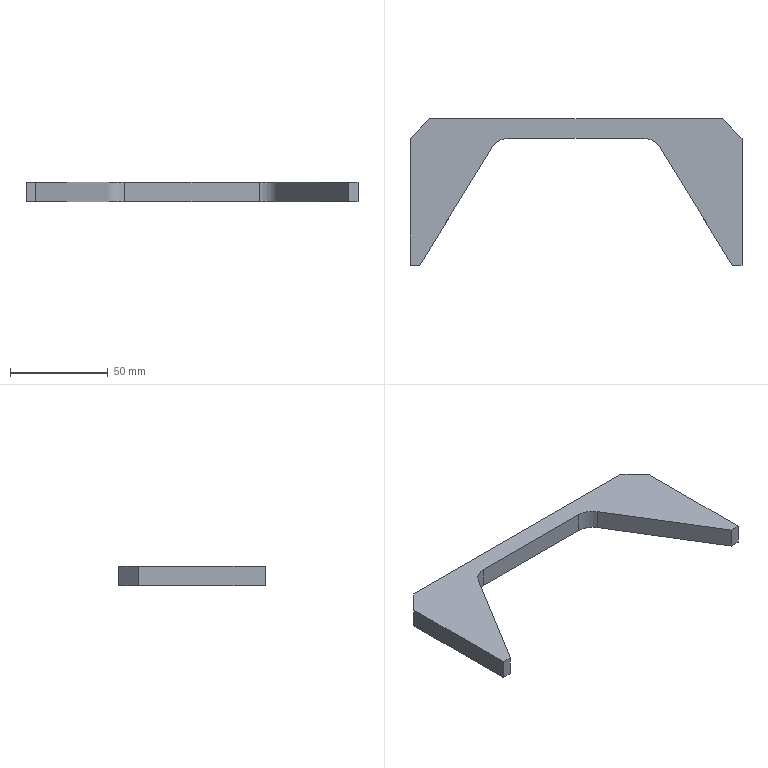Part | SolidWorks | features Chamfer 1, Extrusion 1 | 1 solid | 14 faces | box 170 x 75 x 10 mm | volume 48537 mm3 | plane 12 | cylinder 2 | commonest cylinder face diameters 20 x2
STEP:
#1=CARTESIAN_POINT('',(-85.,65.,5.));
#2=VERTEX_POINT('',#1);
#3=CARTESIAN_POINT('',(-85.,0.,5.));
#4=VERTEX_POINT('',#3);
#5=CARTESIAN_POINT('',(-85.,75.,5.));
#6=DIRECTION('',(0.,-1.,0.));
#7=VECTOR('',#6,1000.);
#8=LINE('',#5,#7);
#9=EDGE_CURVE('',#2,#4,#8,.T.);
#10=ORIENTED_EDGE('',*,*,#9,.F.);
#11=CARTESIAN_POINT('',(-85.,65.,-5.));
#12=VERTEX_POINT('',#11);
#13=CARTESIAN_POINT('',(-85.,65.,5.));
#14=DIRECTION('',(0.,0.,-1.));
#15=VECTOR('',#14,1000.);
#16=LINE('',#13,#15);
#17=EDGE_CURVE('',#2,#12,#16,.T.);
#18=ORIENTED_EDGE('',*,*,#17,.T.);
#19=CARTESIAN_POINT('',(-85.,0.,-5.));
#20=VERTEX_POINT('',#19);
#21=CARTESIAN_POINT('',(-85.,75.,-5.));
#22=DIRECTION('',(0.,-1.,0.));
#23=VECTOR('',#22,1000.);
#24=LINE('',#21,#23);
#25=EDGE_CURVE('',#12,#20,#24,.T.);
#26=ORIENTED_EDGE('',*,*,#25,.T.);
#27=CARTESIAN_POINT('',(-85.,0.,5.));
#28=DIRECTION('',(0.,0.,-1.));
#29=VECTOR('',#28,1000.);
#30=LINE('',#27,#29);
#31=EDGE_CURVE('',#4,#20,#30,.T.);
#32=ORIENTED_EDGE('',*,*,#31,.F.);
#33=EDGE_LOOP('',(#10,#18,#26,#32));
#34=FACE_OUTER_BOUND('',#33,.T.);
#35=CARTESIAN_POINT('',(-85.,75.,5.));
#36=DIRECTION('',(1.,0.,0.));
#37=DIRECTION('',(0.,0.,-1.));
#38=AXIS2_PLACEMENT_3D('',#35,#36,#37);
#39=PLANE('',#38);
#40=ADVANCED_FACE('',(#34),#39,.F.);
#41=CARTESIAN_POINT('',(-80.,0.,-5.));
#42=VERTEX_POINT('',#41);
#43=CARTESIAN_POINT('',(-85.,0.,-5.));
#44=DIRECTION('',(1.,0.,0.));
#45=VECTOR('',#44,1000.);
#46=LINE('',#43,#45);
#47=EDGE_CURVE('',#20,#42,#46,.T.);
#48=ORIENTED_EDGE('',*,*,#47,.T.);
#49=CARTESIAN_POINT('',(-80.,0.,5.));
#50=VERTEX_POINT('',#49);
#51=CARTESIAN_POINT('',(-80.,0.,5.));
#52=DIRECTION('',(0.,0.,-1.));
#53=VECTOR('',#52,1000.);
#54=LINE('',#51,#53);
#55=EDGE_CURVE('',#50,#42,#54,.T.);
#56=ORIENTED_EDGE('',*,*,#55,.F.);
#57=CARTESIAN_POINT('',(-85.,0.,5.));
#58=DIRECTION('',(1.,0.,0.));
#59=VECTOR('',#58,1000.);
#60=LINE('',#57,#59);
#61=EDGE_CURVE('',#4,#50,#60,.T.);
#62=ORIENTED_EDGE('',*,*,#61,.F.);
#63=ORIENTED_EDGE('',*,*,#31,.T.);
#64=EDGE_LOOP('',(#48,#56,#62,#63));
#65=FACE_OUTER_BOUND('',#64,.T.);
#66=CARTESIAN_POINT('',(-85.,0.,5.));
#67=DIRECTION('',(0.,1.,0.));
#68=DIRECTION('',(0.,0.,1.));
#69=AXIS2_PLACEMENT_3D('',#66,#67,#68);
#70=PLANE('',#69);
#71=ADVANCED_FACE('',(#65),#70,.F.);
#72=CARTESIAN_POINT('',(-43.022,60.232,-5.));
#73=VERTEX_POINT('',#72);
#74=CARTESIAN_POINT('',(-80.,0.,-5.));
#75=DIRECTION('',(0.5232,0.8522,0.));
#76=VECTOR('',#75,1000.);
#77=LINE('',#74,#76);
#78=EDGE_CURVE('',#42,#73,#77,.T.);
#79=ORIENTED_EDGE('',*,*,#78,.T.);
#80=CARTESIAN_POINT('',(-43.022,60.232,5.));
#81=VERTEX_POINT('',#80);
#82=CARTESIAN_POINT('',(-43.022,60.232,5.));
#83=DIRECTION('',(0.,0.,-1.));
#84=VECTOR('',#83,1000.);
#85=LINE('',#82,#84);
#86=EDGE_CURVE('',#81,#73,#85,.T.);
#87=ORIENTED_EDGE('',*,*,#86,.F.);
#88=CARTESIAN_POINT('',(-80.,0.,5.));
#89=DIRECTION('',(0.5232,0.8522,0.));
#90=VECTOR('',#89,1000.);
#91=LINE('',#88,#90);
#92=EDGE_CURVE('',#50,#81,#91,.T.);
#93=ORIENTED_EDGE('',*,*,#92,.F.);
#94=ORIENTED_EDGE('',*,*,#55,.T.);
#95=EDGE_LOOP('',(#79,#87,#93,#94));
#96=FACE_OUTER_BOUND('',#95,.T.);
#97=CARTESIAN_POINT('',(-80.,0.,5.));
#98=DIRECTION('',(-0.8522,0.5232,0.));
#99=DIRECTION('',(-0.5232,-0.8522,0.));
#100=AXIS2_PLACEMENT_3D('',#97,#98,#99);
#101=PLANE('',#100);
#102=ADVANCED_FACE('',(#96),#101,.F.);
#103=CARTESIAN_POINT('',(-34.5,65.,-5.));
#104=VERTEX_POINT('',#103);
#105=CARTESIAN_POINT('',(-34.5,55.,-5.));
#106=DIRECTION('',(0.,0.,-1.));
#107=DIRECTION('',(-1.,0.,0.));
#108=AXIS2_PLACEMENT_3D('',#105,#106,#107);
#109=CIRCLE('',#108,10.);
#110=EDGE_CURVE('',#73,#104,#109,.T.);
#111=ORIENTED_EDGE('',*,*,#110,.T.);
#112=CARTESIAN_POINT('',(-34.5,65.,5.));
#113=VERTEX_POINT('',#112);
#114=CARTESIAN_POINT('',(-34.5,65.,5.));
#115=DIRECTION('',(0.,0.,-1.));
#116=VECTOR('',#115,1000.);
#117=LINE('',#114,#116);
#118=EDGE_CURVE('',#113,#104,#117,.T.);
#119=ORIENTED_EDGE('',*,*,#118,.F.);
#120=CARTESIAN_POINT('',(-34.5,55.,5.));
#121=DIRECTION('',(0.,0.,-1.));
#122=DIRECTION('',(-1.,0.,0.));
#123=AXIS2_PLACEMENT_3D('',#120,#121,#122);
#124=CIRCLE('',#123,10.);
#125=EDGE_CURVE('',#81,#113,#124,.T.);
#126=ORIENTED_EDGE('',*,*,#125,.F.);
#127=ORIENTED_EDGE('',*,*,#86,.T.);
#128=EDGE_LOOP('',(#111,#119,#126,#127));
#129=FACE_OUTER_BOUND('',#128,.T.);
#130=CARTESIAN_POINT('',(-34.5,55.,5.));
#131=DIRECTION('',(0.,0.,-1.));
#132=DIRECTION('',(-1.,0.,0.));
#133=AXIS2_PLACEMENT_3D('',#130,#131,#132);
#134=CYLINDRICAL_SURFACE('',#133,10.);
#135=ADVANCED_FACE('',(#129),#134,.F.);
#136=CARTESIAN_POINT('',(34.5,65.,-5.));
#137=VERTEX_POINT('',#136);
#138=CARTESIAN_POINT('',(-34.5,65.,-5.));
#139=DIRECTION('',(1.,0.,0.));
#140=VECTOR('',#139,1000.);
#141=LINE('',#138,#140);
#142=EDGE_CURVE('',#104,#137,#141,.T.);
#143=ORIENTED_EDGE('',*,*,#142,.T.);
#144=CARTESIAN_POINT('',(34.5,65.,5.));
#145=VERTEX_POINT('',#144);
#146=CARTESIAN_POINT('',(34.5,65.,5.));
#147=DIRECTION('',(0.,0.,-1.));
#148=VECTOR('',#147,1000.);
#149=LINE('',#146,#148);
#150=EDGE_CURVE('',#145,#137,#149,.T.);
#151=ORIENTED_EDGE('',*,*,#150,.F.);
#152=CARTESIAN_POINT('',(-34.5,65.,5.));
#153=DIRECTION('',(1.,0.,0.));
#154=VECTOR('',#153,1000.);
#155=LINE('',#152,#154);
#156=EDGE_CURVE('',#113,#145,#155,.T.);
#157=ORIENTED_EDGE('',*,*,#156,.F.);
#158=ORIENTED_EDGE('',*,*,#118,.T.);
#159=EDGE_LOOP('',(#143,#151,#157,#158));
#160=FACE_OUTER_BOUND('',#159,.T.);
#161=CARTESIAN_POINT('',(-34.5,65.,5.));
#162=DIRECTION('',(0.,1.,0.));
#163=DIRECTION('',(0.,0.,1.));
#164=AXIS2_PLACEMENT_3D('',#161,#162,#163);
#165=PLANE('',#164);
#166=ADVANCED_FACE('',(#160),#165,.F.);
#167=CARTESIAN_POINT('',(43.022,60.232,-5.));
#168=VERTEX_POINT('',#167);
#169=CARTESIAN_POINT('',(34.5,55.,-5.));
#170=DIRECTION('',(0.,0.,-1.));
#171=DIRECTION('',(1.,0.,0.));
#172=AXIS2_PLACEMENT_3D('',#169,#170,#171);
#173=CIRCLE('',#172,10.);
#174=EDGE_CURVE('',#137,#168,#173,.T.);
#175=ORIENTED_EDGE('',*,*,#174,.T.);
#176=CARTESIAN_POINT('',(43.022,60.232,5.));
#177=VERTEX_POINT('',#176);
#178=CARTESIAN_POINT('',(43.022,60.232,5.));
#179=DIRECTION('',(0.,0.,-1.));
#180=VECTOR('',#179,1000.);
#181=LINE('',#178,#180);
#182=EDGE_CURVE('',#177,#168,#181,.T.);
#183=ORIENTED_EDGE('',*,*,#182,.F.);
#184=CARTESIAN_POINT('',(34.5,55.,5.));
#185=DIRECTION('',(0.,0.,-1.));
#186=DIRECTION('',(1.,0.,0.));
#187=AXIS2_PLACEMENT_3D('',#184,#185,#186);
#188=CIRCLE('',#187,10.);
#189=EDGE_CURVE('',#145,#177,#188,.T.);
#190=ORIENTED_EDGE('',*,*,#189,.F.);
#191=ORIENTED_EDGE('',*,*,#150,.T.);
#192=EDGE_LOOP('',(#175,#183,#190,#191));
#193=FACE_OUTER_BOUND('',#192,.T.);
#194=CARTESIAN_POINT('',(34.5,55.,5.));
#195=DIRECTION('',(0.,0.,-1.));
#196=DIRECTION('',(-1.,0.,0.));
#197=AXIS2_PLACEMENT_3D('',#194,#195,#196);
#198=CYLINDRICAL_SURFACE('',#197,10.);
#199=ADVANCED_FACE('',(#193),#198,.F.);
#200=CARTESIAN_POINT('',(80.,0.,-5.));
#201=VERTEX_POINT('',#200);
#202=CARTESIAN_POINT('',(80.,0.,-5.));
#203=DIRECTION('',(0.5232,-0.8522,0.));
#204=VECTOR('',#203,1000.);
#205=LINE('',#202,#204);
#206=EDGE_CURVE('',#168,#201,#205,.T.);
#207=ORIENTED_EDGE('',*,*,#206,.T.);
#208=CARTESIAN_POINT('',(80.,0.,5.));
#209=VERTEX_POINT('',#208);
#210=CARTESIAN_POINT('',(80.,0.,5.));
#211=DIRECTION('',(0.,0.,-1.));
#212=VECTOR('',#211,1000.);
#213=LINE('',#210,#212);
#214=EDGE_CURVE('',#209,#201,#213,.T.);
#215=ORIENTED_EDGE('',*,*,#214,.F.);
#216=CARTESIAN_POINT('',(80.,0.,5.));
#217=DIRECTION('',(0.5232,-0.8522,0.));
#218=VECTOR('',#217,1000.);
#219=LINE('',#216,#218);
#220=EDGE_CURVE('',#177,#209,#219,.T.);
#221=ORIENTED_EDGE('',*,*,#220,.F.);
#222=ORIENTED_EDGE('',*,*,#182,.T.);
#223=EDGE_LOOP('',(#207,#215,#221,#222));
#224=FACE_OUTER_BOUND('',#223,.T.);
#225=CARTESIAN_POINT('',(80.,0.,5.));
#226=DIRECTION('',(0.8522,0.5232,0.));
#227=DIRECTION('',(-0.5232,0.8522,0.));
#228=AXIS2_PLACEMENT_3D('',#225,#226,#227);
#229=PLANE('',#228);
#230=ADVANCED_FACE('',(#224),#229,.F.);
#231=CARTESIAN_POINT('',(85.,0.,-5.));
#232=VERTEX_POINT('',#231);
#233=CARTESIAN_POINT('',(85.,0.,-5.));
#234=DIRECTION('',(1.,0.,0.));
#235=VECTOR('',#234,1000.);
#236=LINE('',#233,#235);
#237=EDGE_CURVE('',#201,#232,#236,.T.);
#238=ORIENTED_EDGE('',*,*,#237,.T.);
#239=CARTESIAN_POINT('',(85.,0.,5.));
#240=VERTEX_POINT('',#239);
#241=CARTESIAN_POINT('',(85.,0.,5.));
#242=DIRECTION('',(0.,0.,-1.));
#243=VECTOR('',#242,1000.);
#244=LINE('',#241,#243);
#245=EDGE_CURVE('',#240,#232,#244,.T.);
#246=ORIENTED_EDGE('',*,*,#245,.F.);
#247=CARTESIAN_POINT('',(85.,0.,5.));
#248=DIRECTION('',(1.,0.,0.));
#249=VECTOR('',#248,1000.);
#250=LINE('',#247,#249);
#251=EDGE_CURVE('',#209,#240,#250,.T.);
#252=ORIENTED_EDGE('',*,*,#251,.F.);
#253=ORIENTED_EDGE('',*,*,#214,.T.);
#254=EDGE_LOOP('',(#238,#246,#252,#253));
#255=FACE_OUTER_BOUND('',#254,.T.);
#256=CARTESIAN_POINT('',(85.,0.,5.));
#257=DIRECTION('',(0.,1.,0.));
#258=DIRECTION('',(0.,0.,1.));
#259=AXIS2_PLACEMENT_3D('',#256,#257,#258);
#260=PLANE('',#259);
#261=ADVANCED_FACE('',(#255),#260,.F.);
#262=CARTESIAN_POINT('',(85.,65.,-5.));
#263=VERTEX_POINT('',#262);
#264=CARTESIAN_POINT('',(85.,75.,-5.));
#265=DIRECTION('',(0.,1.,0.));
#266=VECTOR('',#265,1000.);
#267=LINE('',#264,#266);
#268=EDGE_CURVE('',#232,#263,#267,.T.);
#269=ORIENTED_EDGE('',*,*,#268,.T.);
#270=CARTESIAN_POINT('',(85.,65.,5.));
#271=VERTEX_POINT('',#270);
#272=CARTESIAN_POINT('',(85.,65.,5.));
#273=DIRECTION('',(0.,0.,1.));
#274=VECTOR('',#273,1000.);
#275=LINE('',#272,#274);
#276=EDGE_CURVE('',#263,#271,#275,.T.);
#277=ORIENTED_EDGE('',*,*,#276,.T.);
#278=CARTESIAN_POINT('',(85.,75.,5.));
#279=DIRECTION('',(0.,1.,0.));
#280=VECTOR('',#279,1000.);
#281=LINE('',#278,#280);
#282=EDGE_CURVE('',#240,#271,#281,.T.);
#283=ORIENTED_EDGE('',*,*,#282,.F.);
#284=ORIENTED_EDGE('',*,*,#245,.T.);
#285=EDGE_LOOP('',(#269,#277,#283,#284));
#286=FACE_OUTER_BOUND('',#285,.T.);
#287=CARTESIAN_POINT('',(85.,75.,5.));
#288=DIRECTION('',(-1.,0.,0.));
#289=DIRECTION('',(0.,0.,1.));
#290=AXIS2_PLACEMENT_3D('',#287,#288,#289);
#291=PLANE('',#290);
#292=ADVANCED_FACE('',(#286),#291,.F.);
#293=CARTESIAN_POINT('',(75.,75.,5.));
#294=VERTEX_POINT('',#293);
#295=CARTESIAN_POINT('',(-75.,75.,5.));
#296=VERTEX_POINT('',#295);
#297=CARTESIAN_POINT('',(85.,75.,5.));
#298=DIRECTION('',(-1.,0.,0.));
#299=VECTOR('',#298,1000.);
#300=LINE('',#297,#299);
#301=EDGE_CURVE('',#294,#296,#300,.T.);
#302=ORIENTED_EDGE('',*,*,#301,.F.);
#303=CARTESIAN_POINT('',(75.,75.,-5.));
#304=VERTEX_POINT('',#303);
#305=CARTESIAN_POINT('',(75.,75.,5.));
#306=DIRECTION('',(0.,0.,-1.));
#307=VECTOR('',#306,1000.);
#308=LINE('',#305,#307);
#309=EDGE_CURVE('',#294,#304,#308,.T.);
#310=ORIENTED_EDGE('',*,*,#309,.T.);
#311=CARTESIAN_POINT('',(-75.,75.,-5.));
#312=VERTEX_POINT('',#311);
#313=CARTESIAN_POINT('',(85.,75.,-5.));
#314=DIRECTION('',(-1.,0.,0.));
#315=VECTOR('',#314,1000.);
#316=LINE('',#313,#315);
#317=EDGE_CURVE('',#304,#312,#316,.T.);
#318=ORIENTED_EDGE('',*,*,#317,.T.);
#319=CARTESIAN_POINT('',(-75.,75.,5.));
#320=DIRECTION('',(0.,0.,1.));
#321=VECTOR('',#320,1000.);
#322=LINE('',#319,#321);
#323=EDGE_CURVE('',#312,#296,#322,.T.);
#324=ORIENTED_EDGE('',*,*,#323,.T.);
#325=EDGE_LOOP('',(#302,#310,#318,#324));
#326=FACE_OUTER_BOUND('',#325,.T.);
#327=CARTESIAN_POINT('',(85.,75.,5.));
#328=DIRECTION('',(0.,-1.,0.));
#329=DIRECTION('',(1.,0.,0.));
#330=AXIS2_PLACEMENT_3D('',#327,#328,#329);
#331=PLANE('',#330);
#332=ADVANCED_FACE('',(#326),#331,.F.);
#333=ORIENTED_EDGE('',*,*,#282,.T.);
#334=CARTESIAN_POINT('',(75.,75.,5.));
#335=DIRECTION('',(-0.7071,0.7071,0.));
#336=VECTOR('',#335,1000.);
#337=LINE('',#334,#336);
#338=EDGE_CURVE('',#271,#294,#337,.T.);
#339=ORIENTED_EDGE('',*,*,#338,.T.);
#340=ORIENTED_EDGE('',*,*,#301,.T.);
#341=CARTESIAN_POINT('',(-85.,65.,5.));
#342=DIRECTION('',(-0.7071,-0.7071,0.));
#343=VECTOR('',#342,1000.);
#344=LINE('',#341,#343);
#345=EDGE_CURVE('',#296,#2,#344,.T.);
#346=ORIENTED_EDGE('',*,*,#345,.T.);
#347=ORIENTED_EDGE('',*,*,#9,.T.);
#348=ORIENTED_EDGE('',*,*,#61,.T.);
#349=ORIENTED_EDGE('',*,*,#92,.T.);
#350=ORIENTED_EDGE('',*,*,#125,.T.);
#351=ORIENTED_EDGE('',*,*,#156,.T.);
#352=ORIENTED_EDGE('',*,*,#189,.T.);
#353=ORIENTED_EDGE('',*,*,#220,.T.);
#354=ORIENTED_EDGE('',*,*,#251,.T.);
#355=EDGE_LOOP('',(#333,#339,#340,#346,#347,#348,#349,#350,#351,#352,#353,#354));
#356=FACE_OUTER_BOUND('',#355,.T.);
#357=CARTESIAN_POINT('',(-34.5,55.,5.));
#358=DIRECTION('',(0.,0.,-1.));
#359=DIRECTION('',(-1.,0.,0.));
#360=AXIS2_PLACEMENT_3D('',#357,#358,#359);
#361=PLANE('',#360);
#362=ADVANCED_FACE('',(#356),#361,.F.);
#363=ORIENTED_EDGE('',*,*,#317,.F.);
#364=CARTESIAN_POINT('',(30.25,119.75,-5.));
#365=DIRECTION('',(0.7071,-0.7071,0.));
#366=VECTOR('',#365,1000.);
#367=LINE('',#364,#366);
#368=EDGE_CURVE('',#304,#263,#367,.T.);
#369=ORIENTED_EDGE('',*,*,#368,.T.);
#370=ORIENTED_EDGE('',*,*,#268,.F.);
#371=ORIENTED_EDGE('',*,*,#237,.F.);
#372=ORIENTED_EDGE('',*,*,#206,.F.);
#373=ORIENTED_EDGE('',*,*,#174,.F.);
#374=ORIENTED_EDGE('',*,*,#142,.F.);
#375=ORIENTED_EDGE('',*,*,#110,.F.);
#376=ORIENTED_EDGE('',*,*,#78,.F.);
#377=ORIENTED_EDGE('',*,*,#47,.F.);
#378=ORIENTED_EDGE('',*,*,#25,.F.);
#379=CARTESIAN_POINT('',(-64.75,85.25,-5.));
#380=DIRECTION('',(0.7071,0.7071,0.));
#381=VECTOR('',#380,1000.);
#382=LINE('',#379,#381);
#383=EDGE_CURVE('',#12,#312,#382,.T.);
#384=ORIENTED_EDGE('',*,*,#383,.T.);
#385=EDGE_LOOP('',(#363,#369,#370,#371,#372,#373,#374,#375,#376,#377,#378,#384));
#386=FACE_OUTER_BOUND('',#385,.T.);
#387=CARTESIAN_POINT('',(-34.5,55.,-5.));
#388=DIRECTION('',(0.,0.,-1.));
#389=DIRECTION('',(-1.,0.,0.));
#390=AXIS2_PLACEMENT_3D('',#387,#388,#389);
#391=PLANE('',#390);
#392=ADVANCED_FACE('',(#386),#391,.T.);
#393=ORIENTED_EDGE('',*,*,#338,.F.);
#394=ORIENTED_EDGE('',*,*,#276,.F.);
#395=ORIENTED_EDGE('',*,*,#368,.F.);
#396=ORIENTED_EDGE('',*,*,#309,.F.);
#397=EDGE_LOOP('',(#393,#394,#395,#396));
#398=FACE_OUTER_BOUND('',#397,.T.);
#399=CARTESIAN_POINT('',(75.,75.,5.));
#400=DIRECTION('',(-0.7071,-0.7071,0.));
#401=DIRECTION('',(0.,0.,-1.));
#402=AXIS2_PLACEMENT_3D('',#399,#400,#401);
#403=PLANE('',#402);
#404=ADVANCED_FACE('',(#398),#403,.F.);
#405=ORIENTED_EDGE('',*,*,#345,.F.);
#406=ORIENTED_EDGE('',*,*,#323,.F.);
#407=ORIENTED_EDGE('',*,*,#383,.F.);
#408=ORIENTED_EDGE('',*,*,#17,.F.);
#409=EDGE_LOOP('',(#405,#406,#407,#408));
#410=FACE_OUTER_BOUND('',#409,.T.);
#411=CARTESIAN_POINT('',(-85.,65.,5.));
#412=DIRECTION('',(0.7071,-0.7071,0.));
#413=DIRECTION('',(0.,0.,-1.));
#414=AXIS2_PLACEMENT_3D('',#411,#412,#413);
#415=PLANE('',#414);
#416=ADVANCED_FACE('',(#410),#415,.F.);
#417=CLOSED_SHELL('',(#40,#71,#102,#135,#166,#199,#230,#261,#292,#332,#362,#392,#404,#416));
#418=MANIFOLD_SOLID_BREP('',#417);
#419=CARTESIAN_POINT('',(0.,0.,0.));
#420=DIRECTION('',(0.,0.,1.));
#421=DIRECTION('',(1.,0.,0.));
#422=AXIS2_PLACEMENT_3D('',#419,#420,#421);
#423=(LENGTH_UNIT()NAMED_UNIT(*)SI_UNIT(.MILLI.,.METRE.));
#424=UNCERTAINTY_MEASURE_WITH_UNIT(LENGTH_MEASURE(0.00001),#423,'','');
#425=(NAMED_UNIT(*)PLANE_ANGLE_UNIT()SI_UNIT($,.RADIAN.));
#426=(NAMED_UNIT(*)SI_UNIT($,.STERADIAN.)SOLID_ANGLE_UNIT());
#427=(GEOMETRIC_REPRESENTATION_CONTEXT(3)GLOBAL_UNCERTAINTY_ASSIGNED_CONTEXT((#424))GLOBAL_UNIT_ASSIGNED_CONTEXT((#423,#425,#426))REPRESENTATION_CONTEXT('',''));
#428=ADVANCED_BREP_SHAPE_REPRESENTATION('',(#418,#422),#427);